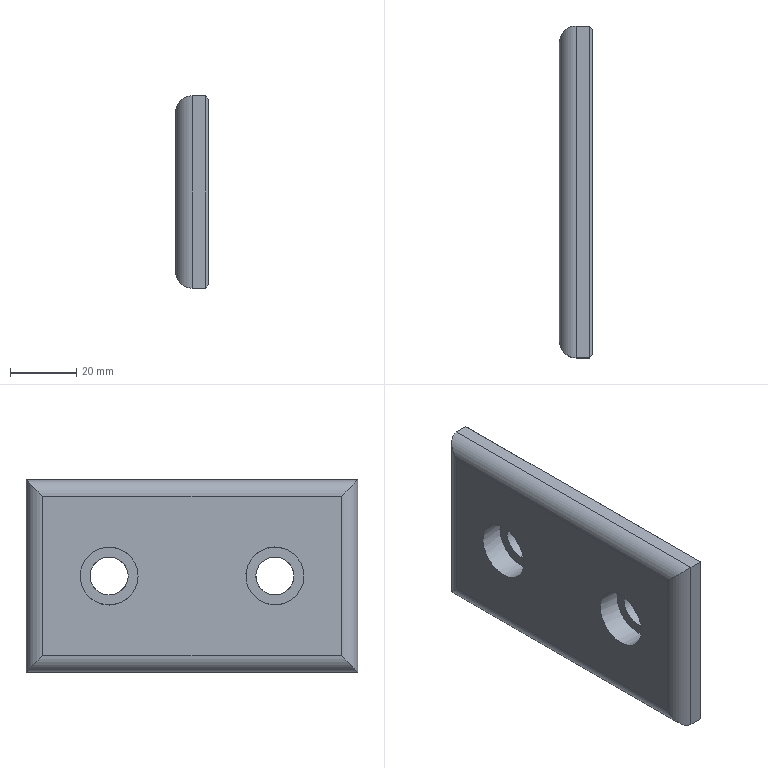Part | NX | features solid 2 | 1 solid | 20 faces | box 10 x 100 x 58 mm | volume 52123 mm3 | plane 12 | cylinder 8 | commonest cylinder face diameters 10 x4 11.5 x2 17.5 x2
STEP:
#1=CARTESIAN_POINT('',(-1316.,-845.,-345.));
#2=VERTEX_POINT('',#1);
#3=CARTESIAN_POINT('',(-1320.,-845.,-345.));
#4=VERTEX_POINT('',#3);
#5=CARTESIAN_POINT('',(-1315.,-845.,-345.));
#6=DIRECTION('',(-1.,0.,0.));
#7=VECTOR('',#6,1000.);
#8=LINE('',#5,#7);
#9=EDGE_CURVE('',#2,#4,#8,.T.);
#10=ORIENTED_EDGE('',*,*,#9,.F.);
#11=CARTESIAN_POINT('',(-1316.,-845.,-287.));
#12=VERTEX_POINT('',#11);
#13=CARTESIAN_POINT('',(-1316.,-845.,-287.));
#14=DIRECTION('',(0.,0.,1.));
#15=VECTOR('',#14,1000.);
#16=LINE('',#13,#15);
#17=EDGE_CURVE('',#2,#12,#16,.T.);
#18=ORIENTED_EDGE('',*,*,#17,.T.);
#19=CARTESIAN_POINT('',(-1320.,-845.,-287.));
#20=VERTEX_POINT('',#19);
#21=CARTESIAN_POINT('',(-1315.,-845.,-287.));
#22=DIRECTION('',(-1.,0.,0.));
#23=VECTOR('',#22,1000.);
#24=LINE('',#21,#23);
#25=EDGE_CURVE('',#12,#20,#24,.T.);
#26=ORIENTED_EDGE('',*,*,#25,.T.);
#27=CARTESIAN_POINT('',(-1320.,-845.,-345.));
#28=DIRECTION('',(0.,0.,-1.));
#29=VECTOR('',#28,1000.);
#30=LINE('',#27,#29);
#31=EDGE_CURVE('',#20,#4,#30,.T.);
#32=ORIENTED_EDGE('',*,*,#31,.T.);
#33=EDGE_LOOP('',(#10,#18,#26,#32));
#34=FACE_BOUND('',#33,.T.);
#35=CARTESIAN_POINT('',(-1315.,-845.,-287.));
#36=DIRECTION('',(0.,1.,0.));
#37=DIRECTION('',(0.,0.,-1.));
#38=AXIS2_PLACEMENT_3D('',#35,#36,#37);
#39=PLANE('',#38);
#40=ADVANCED_FACE('',(#34),#39,.F.);
#41=CARTESIAN_POINT('',(-1316.,-745.,-345.));
#42=VERTEX_POINT('',#41);
#43=CARTESIAN_POINT('',(-1320.,-745.,-345.));
#44=VERTEX_POINT('',#43);
#45=CARTESIAN_POINT('',(-1315.,-745.,-345.));
#46=DIRECTION('',(-1.,0.,0.));
#47=VECTOR('',#46,1000.);
#48=LINE('',#45,#47);
#49=EDGE_CURVE('',#42,#44,#48,.T.);
#50=ORIENTED_EDGE('',*,*,#49,.F.);
#51=CARTESIAN_POINT('',(-1316.,-870.,-345.));
#52=DIRECTION('',(0.,-1.,0.));
#53=VECTOR('',#52,1000.);
#54=LINE('',#51,#53);
#55=EDGE_CURVE('',#42,#2,#54,.T.);
#56=ORIENTED_EDGE('',*,*,#55,.T.);
#57=ORIENTED_EDGE('',*,*,#9,.T.);
#58=CARTESIAN_POINT('',(-1320.,-770.,-345.));
#59=DIRECTION('',(0.,1.,0.));
#60=VECTOR('',#59,1000.);
#61=LINE('',#58,#60);
#62=EDGE_CURVE('',#4,#44,#61,.T.);
#63=ORIENTED_EDGE('',*,*,#62,.T.);
#64=EDGE_LOOP('',(#50,#56,#57,#63));
#65=FACE_BOUND('',#64,.T.);
#66=CARTESIAN_POINT('',(-1315.,-870.,-345.));
#67=DIRECTION('',(0.,0.,1.));
#68=DIRECTION('',(0.,1.,0.));
#69=AXIS2_PLACEMENT_3D('',#66,#67,#68);
#70=PLANE('',#69);
#71=ADVANCED_FACE('',(#65),#70,.F.);
#72=CARTESIAN_POINT('',(-1316.,-745.,-287.));
#73=VERTEX_POINT('',#72);
#74=CARTESIAN_POINT('',(-1320.,-745.,-287.));
#75=VERTEX_POINT('',#74);
#76=CARTESIAN_POINT('',(-1315.,-745.,-287.));
#77=DIRECTION('',(-1.,0.,0.));
#78=VECTOR('',#77,1000.);
#79=LINE('',#76,#78);
#80=EDGE_CURVE('',#73,#75,#79,.T.);
#81=ORIENTED_EDGE('',*,*,#80,.F.);
#82=CARTESIAN_POINT('',(-1316.,-745.,-345.));
#83=DIRECTION('',(0.,0.,-1.));
#84=VECTOR('',#83,1000.);
#85=LINE('',#82,#84);
#86=EDGE_CURVE('',#73,#42,#85,.T.);
#87=ORIENTED_EDGE('',*,*,#86,.T.);
#88=ORIENTED_EDGE('',*,*,#49,.T.);
#89=CARTESIAN_POINT('',(-1320.,-745.,-287.));
#90=DIRECTION('',(0.,0.,1.));
#91=VECTOR('',#90,1000.);
#92=LINE('',#89,#91);
#93=EDGE_CURVE('',#44,#75,#92,.T.);
#94=ORIENTED_EDGE('',*,*,#93,.T.);
#95=EDGE_LOOP('',(#81,#87,#88,#94));
#96=FACE_BOUND('',#95,.T.);
#97=CARTESIAN_POINT('',(-1315.,-745.,-345.));
#98=DIRECTION('',(0.,-1.,0.));
#99=DIRECTION('',(0.,0.,1.));
#100=AXIS2_PLACEMENT_3D('',#97,#98,#99);
#101=PLANE('',#100);
#102=ADVANCED_FACE('',(#96),#101,.F.);
#103=ORIENTED_EDGE('',*,*,#25,.F.);
#104=CARTESIAN_POINT('',(-1316.,-770.,-287.));
#105=DIRECTION('',(0.,1.,0.));
#106=VECTOR('',#105,1000.);
#107=LINE('',#104,#106);
#108=EDGE_CURVE('',#12,#73,#107,.T.);
#109=ORIENTED_EDGE('',*,*,#108,.T.);
#110=ORIENTED_EDGE('',*,*,#80,.T.);
#111=CARTESIAN_POINT('',(-1320.,-870.,-287.));
#112=DIRECTION('',(0.,-1.,0.));
#113=VECTOR('',#112,1000.);
#114=LINE('',#111,#113);
#115=EDGE_CURVE('',#75,#20,#114,.T.);
#116=ORIENTED_EDGE('',*,*,#115,.T.);
#117=EDGE_LOOP('',(#103,#109,#110,#116));
#118=FACE_BOUND('',#117,.T.);
#119=CARTESIAN_POINT('',(-1315.,-770.,-287.));
#120=DIRECTION('',(0.,0.,-1.));
#121=DIRECTION('',(0.,-1.,0.));
#122=AXIS2_PLACEMENT_3D('',#119,#120,#121);
#123=PLANE('',#122);
#124=ADVANCED_FACE('',(#118),#123,.F.);
#125=CARTESIAN_POINT('',(-1315.,-844.,-288.));
#126=VERTEX_POINT('',#125);
#127=CARTESIAN_POINT('',(-1315.,-844.,-344.));
#128=VERTEX_POINT('',#127);
#129=CARTESIAN_POINT('',(-1315.,-844.,-287.));
#130=DIRECTION('',(0.,0.,1.));
#131=VECTOR('',#130,1000.);
#132=LINE('',#129,#131);
#133=EDGE_CURVE('',#126,#128,#132,.F.);
#134=ORIENTED_EDGE('',*,*,#133,.T.);
#135=CARTESIAN_POINT('',(-1315.,-746.,-344.));
#136=VERTEX_POINT('',#135);
#137=CARTESIAN_POINT('',(-1315.,-870.,-344.));
#138=DIRECTION('',(0.,1.,0.));
#139=VECTOR('',#138,1000.);
#140=LINE('',#137,#139);
#141=EDGE_CURVE('',#128,#136,#140,.T.);
#142=ORIENTED_EDGE('',*,*,#141,.T.);
#143=CARTESIAN_POINT('',(-1315.,-746.,-288.));
#144=VERTEX_POINT('',#143);
#145=CARTESIAN_POINT('',(-1315.,-746.,-287.));
#146=DIRECTION('',(0.,0.,-1.));
#147=VECTOR('',#146,1000.);
#148=LINE('',#145,#147);
#149=EDGE_CURVE('',#136,#144,#148,.F.);
#150=ORIENTED_EDGE('',*,*,#149,.T.);
#151=CARTESIAN_POINT('',(-1315.,-870.,-288.));
#152=DIRECTION('',(0.,-1.,0.));
#153=VECTOR('',#152,1000.);
#154=LINE('',#151,#153);
#155=EDGE_CURVE('',#144,#126,#154,.T.);
#156=ORIENTED_EDGE('',*,*,#155,.T.);
#157=EDGE_LOOP('',(#134,#142,#150,#156));
#158=FACE_BOUND('',#157,.T.);
#159=CARTESIAN_POINT('',(-1315.,-770.,-321.75));
#160=VERTEX_POINT('',#159);
#161=CARTESIAN_POINT('',(-1315.,-770.,-316.));
#162=DIRECTION('',(1.,0.,0.));
#163=DIRECTION('',(0.,0.,-1.));
#164=AXIS2_PLACEMENT_3D('',#161,#162,#163);
#165=CIRCLE('',#164,5.75);
#166=EDGE_CURVE('',#160,#160,#165,.F.);
#167=ORIENTED_EDGE('',*,*,#166,.T.);
#168=EDGE_LOOP('',(#167));
#169=FACE_BOUND('',#168,.T.);
#170=CARTESIAN_POINT('',(-1315.,-820.,-310.25));
#171=VERTEX_POINT('',#170);
#172=CARTESIAN_POINT('',(-1315.,-820.,-316.));
#173=DIRECTION('',(1.,0.,0.));
#174=DIRECTION('',(0.,0.,1.));
#175=AXIS2_PLACEMENT_3D('',#172,#173,#174);
#176=CIRCLE('',#175,5.75);
#177=EDGE_CURVE('',#171,#171,#176,.F.);
#178=ORIENTED_EDGE('',*,*,#177,.T.);
#179=EDGE_LOOP('',(#178));
#180=FACE_BOUND('',#179,.T.);
#181=CARTESIAN_POINT('',(-1315.,-870.,-287.));
#182=DIRECTION('',(-1.,0.,0.));
#183=DIRECTION('',(0.,1.,0.));
#184=AXIS2_PLACEMENT_3D('',#181,#182,#183);
#185=PLANE('',#184);
#186=ADVANCED_FACE('',(#158,#169,#180),#185,.F.);
#187=CARTESIAN_POINT('',(-1325.,-750.,-292.));
#188=VERTEX_POINT('',#187);
#189=CARTESIAN_POINT('',(-1325.,-750.,-340.));
#190=VERTEX_POINT('',#189);
#191=CARTESIAN_POINT('',(-1325.,-750.,-287.));
#192=DIRECTION('',(0.,0.,-1.));
#193=VECTOR('',#192,1000.);
#194=LINE('',#191,#193);
#195=EDGE_CURVE('',#188,#190,#194,.T.);
#196=ORIENTED_EDGE('',*,*,#195,.T.);
#197=CARTESIAN_POINT('',(-1325.,-840.,-340.));
#198=VERTEX_POINT('',#197);
#199=CARTESIAN_POINT('',(-1325.,-870.,-340.));
#200=DIRECTION('',(0.,1.,0.));
#201=VECTOR('',#200,1000.);
#202=LINE('',#199,#201);
#203=EDGE_CURVE('',#190,#198,#202,.F.);
#204=ORIENTED_EDGE('',*,*,#203,.T.);
#205=CARTESIAN_POINT('',(-1325.,-840.,-292.));
#206=VERTEX_POINT('',#205);
#207=CARTESIAN_POINT('',(-1325.,-840.,-287.));
#208=DIRECTION('',(0.,0.,1.));
#209=VECTOR('',#208,1000.);
#210=LINE('',#207,#209);
#211=EDGE_CURVE('',#198,#206,#210,.T.);
#212=ORIENTED_EDGE('',*,*,#211,.T.);
#213=CARTESIAN_POINT('',(-1325.,-770.,-292.));
#214=DIRECTION('',(0.,-1.,0.));
#215=VECTOR('',#214,1000.);
#216=LINE('',#213,#215);
#217=EDGE_CURVE('',#206,#188,#216,.F.);
#218=ORIENTED_EDGE('',*,*,#217,.T.);
#219=EDGE_LOOP('',(#196,#204,#212,#218));
#220=FACE_BOUND('',#219,.T.);
#221=CARTESIAN_POINT('',(-1325.,-770.,-324.75));
#222=VERTEX_POINT('',#221);
#223=CARTESIAN_POINT('',(-1325.,-770.,-316.));
#224=DIRECTION('',(1.,0.,0.));
#225=DIRECTION('',(0.,0.,-1.));
#226=AXIS2_PLACEMENT_3D('',#223,#224,#225);
#227=CIRCLE('',#226,8.75);
#228=EDGE_CURVE('',#222,#222,#227,.T.);
#229=ORIENTED_EDGE('',*,*,#228,.T.);
#230=EDGE_LOOP('',(#229));
#231=FACE_BOUND('',#230,.T.);
#232=CARTESIAN_POINT('',(-1325.,-820.,-307.25));
#233=VERTEX_POINT('',#232);
#234=CARTESIAN_POINT('',(-1325.,-820.,-316.));
#235=DIRECTION('',(1.,0.,0.));
#236=DIRECTION('',(0.,0.,1.));
#237=AXIS2_PLACEMENT_3D('',#234,#235,#236);
#238=CIRCLE('',#237,8.75);
#239=EDGE_CURVE('',#233,#233,#238,.T.);
#240=ORIENTED_EDGE('',*,*,#239,.T.);
#241=EDGE_LOOP('',(#240));
#242=FACE_BOUND('',#241,.T.);
#243=CARTESIAN_POINT('',(-1325.,-870.,-287.));
#244=DIRECTION('',(-1.,0.,0.));
#245=DIRECTION('',(0.,1.,0.));
#246=AXIS2_PLACEMENT_3D('',#243,#244,#245);
#247=PLANE('',#246);
#248=ADVANCED_FACE('',(#220,#231,#242),#247,.T.);
#249=CARTESIAN_POINT('',(-1317.7,-825.75,-316.));
#250=VERTEX_POINT('',#249);
#251=CARTESIAN_POINT('',(-1317.7,-820.,-316.));
#252=DIRECTION('',(1.,0.,0.));
#253=DIRECTION('',(0.,-1.,0.));
#254=AXIS2_PLACEMENT_3D('',#251,#252,#253);
#255=CIRCLE('',#254,5.75);
#256=EDGE_CURVE('',#250,#250,#255,.T.);
#257=ORIENTED_EDGE('',*,*,#256,.F.);
#258=EDGE_LOOP('',(#257));
#259=FACE_BOUND('',#258,.T.);
#260=ORIENTED_EDGE('',*,*,#177,.F.);
#261=EDGE_LOOP('',(#260));
#262=FACE_BOUND('',#261,.T.);
#263=CARTESIAN_POINT('',(-1275.,-820.,-316.));
#264=DIRECTION('',(1.,0.,0.));
#265=DIRECTION('',(0.,-1.,0.));
#266=AXIS2_PLACEMENT_3D('',#263,#264,#265);
#267=CYLINDRICAL_SURFACE('',#266,5.75);
#268=ADVANCED_FACE('',(#259,#262),#267,.F.);
#269=ORIENTED_EDGE('',*,*,#256,.T.);
#270=EDGE_LOOP('',(#269));
#271=FACE_BOUND('',#270,.T.);
#272=CARTESIAN_POINT('',(-1317.7,-828.75,-316.));
#273=VERTEX_POINT('',#272);
#274=CARTESIAN_POINT('',(-1317.7,-820.,-316.));
#275=DIRECTION('',(1.,0.,0.));
#276=DIRECTION('',(0.,-1.,0.));
#277=AXIS2_PLACEMENT_3D('',#274,#275,#276);
#278=CIRCLE('',#277,8.75);
#279=EDGE_CURVE('',#273,#273,#278,.T.);
#280=ORIENTED_EDGE('',*,*,#279,.F.);
#281=EDGE_LOOP('',(#280));
#282=FACE_BOUND('',#281,.T.);
#283=CARTESIAN_POINT('',(-1317.7,-820.,-316.));
#284=DIRECTION('',(1.,0.,0.));
#285=DIRECTION('',(0.,-1.,0.));
#286=AXIS2_PLACEMENT_3D('',#283,#284,#285);
#287=PLANE('',#286);
#288=ADVANCED_FACE('',(#271,#282),#287,.F.);
#289=ORIENTED_EDGE('',*,*,#279,.T.);
#290=EDGE_LOOP('',(#289));
#291=FACE_BOUND('',#290,.T.);
#292=ORIENTED_EDGE('',*,*,#239,.F.);
#293=EDGE_LOOP('',(#292));
#294=FACE_BOUND('',#293,.T.);
#295=CARTESIAN_POINT('',(-1325.,-820.,-316.));
#296=DIRECTION('',(1.,0.,0.));
#297=DIRECTION('',(0.,-1.,0.));
#298=AXIS2_PLACEMENT_3D('',#295,#296,#297);
#299=CYLINDRICAL_SURFACE('',#298,8.75);
#300=ADVANCED_FACE('',(#291,#294),#299,.F.);
#301=CARTESIAN_POINT('',(-1317.7,-775.75,-316.));
#302=VERTEX_POINT('',#301);
#303=CARTESIAN_POINT('',(-1317.7,-770.,-316.));
#304=DIRECTION('',(1.,0.,0.));
#305=DIRECTION('',(0.,-1.,0.));
#306=AXIS2_PLACEMENT_3D('',#303,#304,#305);
#307=CIRCLE('',#306,5.75);
#308=EDGE_CURVE('',#302,#302,#307,.T.);
#309=ORIENTED_EDGE('',*,*,#308,.F.);
#310=EDGE_LOOP('',(#309));
#311=FACE_BOUND('',#310,.T.);
#312=ORIENTED_EDGE('',*,*,#166,.F.);
#313=EDGE_LOOP('',(#312));
#314=FACE_BOUND('',#313,.T.);
#315=CARTESIAN_POINT('',(-1275.,-770.,-316.));
#316=DIRECTION('',(1.,0.,0.));
#317=DIRECTION('',(0.,-1.,0.));
#318=AXIS2_PLACEMENT_3D('',#315,#316,#317);
#319=CYLINDRICAL_SURFACE('',#318,5.75);
#320=ADVANCED_FACE('',(#311,#314),#319,.F.);
#321=ORIENTED_EDGE('',*,*,#308,.T.);
#322=EDGE_LOOP('',(#321));
#323=FACE_BOUND('',#322,.T.);
#324=CARTESIAN_POINT('',(-1317.7,-778.75,-316.));
#325=VERTEX_POINT('',#324);
#326=CARTESIAN_POINT('',(-1317.7,-770.,-316.));
#327=DIRECTION('',(1.,0.,0.));
#328=DIRECTION('',(0.,-1.,0.));
#329=AXIS2_PLACEMENT_3D('',#326,#327,#328);
#330=CIRCLE('',#329,8.75);
#331=EDGE_CURVE('',#325,#325,#330,.T.);
#332=ORIENTED_EDGE('',*,*,#331,.F.);
#333=EDGE_LOOP('',(#332));
#334=FACE_BOUND('',#333,.T.);
#335=CARTESIAN_POINT('',(-1317.7,-770.,-316.));
#336=DIRECTION('',(1.,0.,0.));
#337=DIRECTION('',(0.,-1.,0.));
#338=AXIS2_PLACEMENT_3D('',#335,#336,#337);
#339=PLANE('',#338);
#340=ADVANCED_FACE('',(#323,#334),#339,.F.);
#341=ORIENTED_EDGE('',*,*,#331,.T.);
#342=EDGE_LOOP('',(#341));
#343=FACE_BOUND('',#342,.T.);
#344=ORIENTED_EDGE('',*,*,#228,.F.);
#345=EDGE_LOOP('',(#344));
#346=FACE_BOUND('',#345,.T.);
#347=CARTESIAN_POINT('',(-1325.,-770.,-316.));
#348=DIRECTION('',(1.,0.,0.));
#349=DIRECTION('',(0.,-1.,0.));
#350=AXIS2_PLACEMENT_3D('',#347,#348,#349);
#351=CYLINDRICAL_SURFACE('',#350,8.75);
#352=ADVANCED_FACE('',(#343,#346),#351,.F.);
#353=CARTESIAN_POINT('',(-1320.,-750.,-292.));
#354=DIRECTION('',(0.,-0.7071,0.7071));
#355=DIRECTION('',(0.,0.7071,0.7071));
#356=AXIS2_PLACEMENT_3D('',#353,#354,#355);
#357=ELLIPSE('',#356,7.071,5.);
#358=EDGE_CURVE('',#188,#75,#357,.F.);
#359=ORIENTED_EDGE('',*,*,#358,.F.);
#360=ORIENTED_EDGE('',*,*,#217,.F.);
#361=CARTESIAN_POINT('',(-1320.,-840.,-292.));
#362=DIRECTION('',(0.,-0.7071,-0.7071));
#363=DIRECTION('',(0.,0.7071,-0.7071));
#364=AXIS2_PLACEMENT_3D('',#361,#362,#363);
#365=ELLIPSE('',#364,7.071,5.);
#366=EDGE_CURVE('',#20,#206,#365,.T.);
#367=ORIENTED_EDGE('',*,*,#366,.F.);
#368=ORIENTED_EDGE('',*,*,#115,.F.);
#369=EDGE_LOOP('',(#359,#360,#367,#368));
#370=FACE_BOUND('',#369,.T.);
#371=CARTESIAN_POINT('',(-1320.,-770.,-292.));
#372=DIRECTION('',(0.,1.,0.));
#373=DIRECTION('',(0.,0.,-1.));
#374=AXIS2_PLACEMENT_3D('',#371,#372,#373);
#375=CYLINDRICAL_SURFACE('',#374,5.);
#376=ADVANCED_FACE('',(#370),#375,.T.);
#377=ORIENTED_EDGE('',*,*,#366,.T.);
#378=ORIENTED_EDGE('',*,*,#211,.F.);
#379=CARTESIAN_POINT('',(-1320.,-840.,-340.));
#380=DIRECTION('',(0.,0.7071,-0.7071));
#381=DIRECTION('',(0.,0.7071,0.7071));
#382=AXIS2_PLACEMENT_3D('',#379,#380,#381);
#383=ELLIPSE('',#382,7.071,5.);
#384=EDGE_CURVE('',#4,#198,#383,.T.);
#385=ORIENTED_EDGE('',*,*,#384,.F.);
#386=ORIENTED_EDGE('',*,*,#31,.F.);
#387=EDGE_LOOP('',(#377,#378,#385,#386));
#388=FACE_BOUND('',#387,.T.);
#389=CARTESIAN_POINT('',(-1320.,-840.,-287.));
#390=DIRECTION('',(0.,0.,1.));
#391=DIRECTION('',(0.,1.,0.));
#392=AXIS2_PLACEMENT_3D('',#389,#390,#391);
#393=CYLINDRICAL_SURFACE('',#392,5.);
#394=ADVANCED_FACE('',(#388),#393,.T.);
#395=ORIENTED_EDGE('',*,*,#358,.T.);
#396=ORIENTED_EDGE('',*,*,#93,.F.);
#397=CARTESIAN_POINT('',(-1320.,-750.,-340.));
#398=DIRECTION('',(0.,0.7071,0.7071));
#399=DIRECTION('',(0.,0.7071,-0.7071));
#400=AXIS2_PLACEMENT_3D('',#397,#398,#399);
#401=ELLIPSE('',#400,7.071,5.);
#402=EDGE_CURVE('',#190,#44,#401,.F.);
#403=ORIENTED_EDGE('',*,*,#402,.F.);
#404=ORIENTED_EDGE('',*,*,#195,.F.);
#405=EDGE_LOOP('',(#395,#396,#403,#404));
#406=FACE_BOUND('',#405,.T.);
#407=CARTESIAN_POINT('',(-1320.,-750.,-345.));
#408=DIRECTION('',(0.,0.,-1.));
#409=DIRECTION('',(0.,-1.,0.));
#410=AXIS2_PLACEMENT_3D('',#407,#408,#409);
#411=CYLINDRICAL_SURFACE('',#410,5.);
#412=ADVANCED_FACE('',(#406),#411,.T.);
#413=ORIENTED_EDGE('',*,*,#384,.T.);
#414=ORIENTED_EDGE('',*,*,#203,.F.);
#415=ORIENTED_EDGE('',*,*,#402,.T.);
#416=ORIENTED_EDGE('',*,*,#62,.F.);
#417=EDGE_LOOP('',(#413,#414,#415,#416));
#418=FACE_BOUND('',#417,.T.);
#419=CARTESIAN_POINT('',(-1320.,-870.,-340.));
#420=DIRECTION('',(0.,-1.,0.));
#421=DIRECTION('',(0.,0.,1.));
#422=AXIS2_PLACEMENT_3D('',#419,#420,#421);
#423=CYLINDRICAL_SURFACE('',#422,5.);
#424=ADVANCED_FACE('',(#418),#423,.T.);
#425=CARTESIAN_POINT('',(-1273.667,-787.333,-329.333));
#426=DIRECTION('',(0.5774,-0.5774,-0.5774));
#427=VECTOR('',#426,1000.);
#428=LINE('',#425,#427);
#429=EDGE_CURVE('',#73,#144,#428,.T.);
#430=ORIENTED_EDGE('',*,*,#429,.F.);
#431=ORIENTED_EDGE('',*,*,#108,.F.);
#432=CARTESIAN_POINT('',(-1323.667,-852.667,-279.333));
#433=DIRECTION('',(-0.5774,-0.5774,0.5774));
#434=VECTOR('',#433,1000.);
#435=LINE('',#432,#434);
#436=EDGE_CURVE('',#126,#12,#435,.T.);
#437=ORIENTED_EDGE('',*,*,#436,.F.);
#438=ORIENTED_EDGE('',*,*,#155,.F.);
#439=EDGE_LOOP('',(#430,#431,#437,#438));
#440=FACE_BOUND('',#439,.T.);
#441=CARTESIAN_POINT('',(-1315.,-870.,-288.));
#442=DIRECTION('',(-0.7071,0.,-0.7071));
#443=DIRECTION('',(-0.7071,0.,0.7071));
#444=AXIS2_PLACEMENT_3D('',#441,#442,#443);
#445=PLANE('',#444);
#446=ADVANCED_FACE('',(#440),#445,.F.);
#447=ORIENTED_EDGE('',*,*,#436,.T.);
#448=ORIENTED_EDGE('',*,*,#17,.F.);
#449=CARTESIAN_POINT('',(-1296.,-825.,-325.));
#450=DIRECTION('',(-0.5774,-0.5774,-0.5774));
#451=VECTOR('',#450,1000.);
#452=LINE('',#449,#451);
#453=EDGE_CURVE('',#128,#2,#452,.T.);
#454=ORIENTED_EDGE('',*,*,#453,.F.);
#455=ORIENTED_EDGE('',*,*,#133,.F.);
#456=EDGE_LOOP('',(#447,#448,#454,#455));
#457=FACE_BOUND('',#456,.T.);
#458=CARTESIAN_POINT('',(-1315.,-844.,-287.));
#459=DIRECTION('',(-0.7071,0.7071,0.));
#460=DIRECTION('',(0.7071,0.7071,0.));
#461=AXIS2_PLACEMENT_3D('',#458,#459,#460);
#462=PLANE('',#461);
#463=ADVANCED_FACE('',(#457),#462,.F.);
#464=ORIENTED_EDGE('',*,*,#429,.T.);
#465=ORIENTED_EDGE('',*,*,#149,.F.);
#466=CARTESIAN_POINT('',(-1296.,-765.,-325.));
#467=DIRECTION('',(0.5774,-0.5774,0.5774));
#468=VECTOR('',#467,1000.);
#469=LINE('',#466,#468);
#470=EDGE_CURVE('',#42,#136,#469,.T.);
#471=ORIENTED_EDGE('',*,*,#470,.F.);
#472=ORIENTED_EDGE('',*,*,#86,.F.);
#473=EDGE_LOOP('',(#464,#465,#471,#472));
#474=FACE_BOUND('',#473,.T.);
#475=CARTESIAN_POINT('',(-1315.,-746.,-287.));
#476=DIRECTION('',(-0.7071,-0.7071,0.));
#477=DIRECTION('',(-0.7071,0.7071,0.));
#478=AXIS2_PLACEMENT_3D('',#475,#476,#477);
#479=PLANE('',#478);
#480=ADVANCED_FACE('',(#474),#479,.F.);
#481=ORIENTED_EDGE('',*,*,#453,.T.);
#482=ORIENTED_EDGE('',*,*,#55,.F.);
#483=ORIENTED_EDGE('',*,*,#470,.T.);
#484=ORIENTED_EDGE('',*,*,#141,.F.);
#485=EDGE_LOOP('',(#481,#482,#483,#484));
#486=FACE_BOUND('',#485,.T.);
#487=CARTESIAN_POINT('',(-1315.,-870.,-344.));
#488=DIRECTION('',(-0.7071,0.,0.7071));
#489=DIRECTION('',(0.7071,0.,0.7071));
#490=AXIS2_PLACEMENT_3D('',#487,#488,#489);
#491=PLANE('',#490);
#492=ADVANCED_FACE('',(#486),#491,.F.);
#493=CLOSED_SHELL('',(#40,#71,#102,#124,#186,#248,#268,#288,#300,#320,#340,#352,#376,#394,#412,#424,#446,#463,#480,#492));
#494=MANIFOLD_SOLID_BREP('',#493);
#495=(LENGTH_UNIT()NAMED_UNIT(*)SI_UNIT(.MILLI.,.METRE.));
#496=UNCERTAINTY_MEASURE_WITH_UNIT(LENGTH_MEASURE(0.00001),#495,'','');
#497=(NAMED_UNIT(*)PLANE_ANGLE_UNIT()SI_UNIT($,.RADIAN.));
#498=(NAMED_UNIT(*)SI_UNIT($,.STERADIAN.)SOLID_ANGLE_UNIT());
#499=(GEOMETRIC_REPRESENTATION_CONTEXT(3)GLOBAL_UNCERTAINTY_ASSIGNED_CONTEXT((#496))GLOBAL_UNIT_ASSIGNED_CONTEXT((#495,#497,#498))REPRESENTATION_CONTEXT('',''));
#500=ADVANCED_BREP_SHAPE_REPRESENTATION('',(#494),#499);